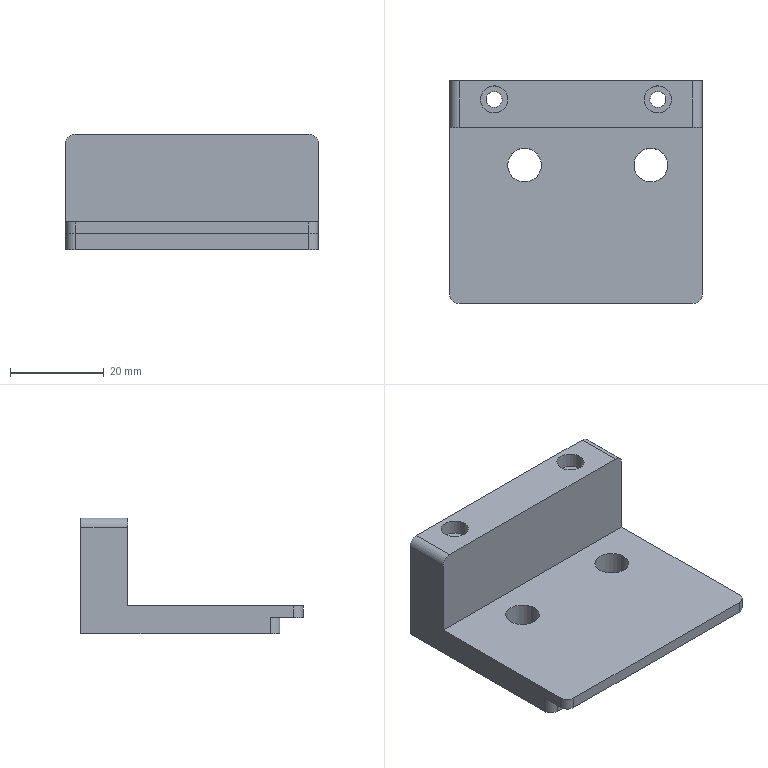Part | STEP file | ROTATION MC_NEW VER-0610_555 | 1 solid | 30 faces | box 54 x 47.54 x 24.76 mm | volume 18101 mm3 | plane 16 | cylinder 14 | commonest cylinder face diameters 4 x6 3 x2 3.4 x2 5.8 x2 7.2 x2
STEP:
#1=CARTESIAN_POINT('',(191.531,578.728,-33.351));
#2=VERTEX_POINT('',#1);
#3=CARTESIAN_POINT('',(193.531,576.728,-33.351));
#4=VERTEX_POINT('',#3);
#5=CARTESIAN_POINT('',(193.531,578.728,-33.351));
#6=DIRECTION('',(0.,0.,1.));
#7=DIRECTION('',(1.,0.,0.));
#8=AXIS2_PLACEMENT_3D('',#5,#6,#7);
#9=CIRCLE('',#8,2.);
#10=EDGE_CURVE('',#2,#4,#9,.T.);
#11=ORIENTED_EDGE('',*,*,#10,.F.);
#12=CARTESIAN_POINT('',(191.531,578.728,-35.851));
#13=VERTEX_POINT('',#12);
#14=CARTESIAN_POINT('',(191.531,578.728,-35.851));
#15=DIRECTION('',(0.,0.,1.));
#16=VECTOR('',#15,2.5);
#17=LINE('',#14,#16);
#18=EDGE_CURVE('',#13,#2,#17,.T.);
#19=ORIENTED_EDGE('',*,*,#18,.F.);
#20=CARTESIAN_POINT('',(193.531,576.728,-35.851));
#21=VERTEX_POINT('',#20);
#22=CARTESIAN_POINT('',(193.531,578.728,-35.851));
#23=DIRECTION('',(0.,0.,-1.));
#24=DIRECTION('',(1.,0.,0.));
#25=AXIS2_PLACEMENT_3D('',#22,#23,#24);
#26=CIRCLE('',#25,2.);
#27=EDGE_CURVE('',#21,#13,#26,.T.);
#28=ORIENTED_EDGE('',*,*,#27,.F.);
#29=CARTESIAN_POINT('',(193.531,576.728,-33.351));
#30=DIRECTION('',(0.,0.,-1.));
#31=VECTOR('',#30,2.5);
#32=LINE('',#29,#31);
#33=EDGE_CURVE('',#4,#21,#32,.T.);
#34=ORIENTED_EDGE('',*,*,#33,.F.);
#35=EDGE_LOOP('',(#11,#19,#28,#34));
#36=FACE_OUTER_BOUND('',#35,.T.);
#37=CARTESIAN_POINT('',(193.531,578.728,-37.851));
#38=DIRECTION('',(0.,0.,1.));
#39=DIRECTION('',(1.,0.,0.));
#40=AXIS2_PLACEMENT_3D('',#37,#38,#39);
#41=CYLINDRICAL_SURFACE('',#40,2.);
#42=ADVANCED_FACE('',(#36),#41,.T.);
#43=CARTESIAN_POINT('',(191.531,583.728,-35.851));
#44=VERTEX_POINT('',#43);
#45=CARTESIAN_POINT('',(193.531,581.728,-35.851));
#46=VERTEX_POINT('',#45);
#47=CARTESIAN_POINT('',(193.531,583.728,-35.851));
#48=DIRECTION('',(0.,0.,1.));
#49=DIRECTION('',(1.,0.,0.));
#50=AXIS2_PLACEMENT_3D('',#47,#48,#49);
#51=CIRCLE('',#50,2.);
#52=EDGE_CURVE('',#44,#46,#51,.T.);
#53=ORIENTED_EDGE('',*,*,#52,.F.);
#54=CARTESIAN_POINT('',(191.531,583.728,-39.351));
#55=VERTEX_POINT('',#54);
#56=CARTESIAN_POINT('',(191.531,583.728,-39.351));
#57=DIRECTION('',(0.,0.,1.));
#58=VECTOR('',#57,3.5);
#59=LINE('',#56,#58);
#60=EDGE_CURVE('',#55,#44,#59,.T.);
#61=ORIENTED_EDGE('',*,*,#60,.F.);
#62=CARTESIAN_POINT('',(193.531,581.728,-39.351));
#63=VERTEX_POINT('',#62);
#64=CARTESIAN_POINT('',(193.531,583.728,-39.351));
#65=DIRECTION('',(0.,0.,-1.));
#66=DIRECTION('',(-1.,0.,0.));
#67=AXIS2_PLACEMENT_3D('',#64,#65,#66);
#68=CIRCLE('',#67,2.);
#69=EDGE_CURVE('',#63,#55,#68,.T.);
#70=ORIENTED_EDGE('',*,*,#69,.F.);
#71=CARTESIAN_POINT('',(193.531,581.728,-35.851));
#72=DIRECTION('',(0.,0.,-1.));
#73=VECTOR('',#72,3.5);
#74=LINE('',#71,#73);
#75=EDGE_CURVE('',#46,#63,#74,.T.);
#76=ORIENTED_EDGE('',*,*,#75,.F.);
#77=EDGE_LOOP('',(#53,#61,#70,#76));
#78=FACE_OUTER_BOUND('',#77,.T.);
#79=CARTESIAN_POINT('',(193.531,583.728,-37.851));
#80=DIRECTION('',(0.,0.,1.));
#81=DIRECTION('',(1.,0.,0.));
#82=AXIS2_PLACEMENT_3D('',#79,#80,#81);
#83=CYLINDRICAL_SURFACE('',#82,2.);
#84=ADVANCED_FACE('',(#78),#83,.T.);
#85=CARTESIAN_POINT('',(243.531,581.728,-35.851));
#86=VERTEX_POINT('',#85);
#87=CARTESIAN_POINT('',(245.531,583.728,-35.851));
#88=VERTEX_POINT('',#87);
#89=CARTESIAN_POINT('',(243.531,583.728,-35.851));
#90=DIRECTION('',(0.,0.,1.));
#91=DIRECTION('',(1.,0.,0.));
#92=AXIS2_PLACEMENT_3D('',#89,#90,#91);
#93=CIRCLE('',#92,2.);
#94=EDGE_CURVE('',#86,#88,#93,.T.);
#95=ORIENTED_EDGE('',*,*,#94,.F.);
#96=CARTESIAN_POINT('',(243.531,581.728,-39.351));
#97=VERTEX_POINT('',#96);
#98=CARTESIAN_POINT('',(243.531,581.728,-39.351));
#99=DIRECTION('',(0.,0.,1.));
#100=VECTOR('',#99,3.5);
#101=LINE('',#98,#100);
#102=EDGE_CURVE('',#97,#86,#101,.T.);
#103=ORIENTED_EDGE('',*,*,#102,.F.);
#104=CARTESIAN_POINT('',(245.531,583.728,-39.351));
#105=VERTEX_POINT('',#104);
#106=CARTESIAN_POINT('',(243.531,583.728,-39.351));
#107=DIRECTION('',(0.,0.,-1.));
#108=DIRECTION('',(-1.,0.,0.));
#109=AXIS2_PLACEMENT_3D('',#106,#107,#108);
#110=CIRCLE('',#109,2.);
#111=EDGE_CURVE('',#105,#97,#110,.T.);
#112=ORIENTED_EDGE('',*,*,#111,.F.);
#113=CARTESIAN_POINT('',(245.531,583.728,-35.851));
#114=DIRECTION('',(0.,0.,-1.));
#115=VECTOR('',#114,3.5);
#116=LINE('',#113,#115);
#117=EDGE_CURVE('',#88,#105,#116,.T.);
#118=ORIENTED_EDGE('',*,*,#117,.F.);
#119=EDGE_LOOP('',(#95,#103,#112,#118));
#120=FACE_OUTER_BOUND('',#119,.T.);
#121=CARTESIAN_POINT('',(243.531,583.728,-17.301));
#122=DIRECTION('',(0.,0.,1.));
#123=DIRECTION('',(1.,0.,0.));
#124=AXIS2_PLACEMENT_3D('',#121,#122,#123);
#125=CYLINDRICAL_SURFACE('',#124,2.);
#126=ADVANCED_FACE('',(#120),#125,.T.);
#127=CARTESIAN_POINT('',(245.531,578.728,-35.851));
#128=VERTEX_POINT('',#127);
#129=CARTESIAN_POINT('',(243.531,576.728,-35.851));
#130=VERTEX_POINT('',#129);
#131=CARTESIAN_POINT('',(243.531,578.728,-35.851));
#132=DIRECTION('',(0.,0.,-1.));
#133=DIRECTION('',(1.,0.,0.));
#134=AXIS2_PLACEMENT_3D('',#131,#132,#133);
#135=CIRCLE('',#134,2.);
#136=EDGE_CURVE('',#128,#130,#135,.T.);
#137=ORIENTED_EDGE('',*,*,#136,.F.);
#138=CARTESIAN_POINT('',(245.531,578.728,-33.351));
#139=VERTEX_POINT('',#138);
#140=CARTESIAN_POINT('',(245.531,578.728,-33.351));
#141=DIRECTION('',(0.,0.,-1.));
#142=VECTOR('',#141,2.5);
#143=LINE('',#140,#142);
#144=EDGE_CURVE('',#139,#128,#143,.T.);
#145=ORIENTED_EDGE('',*,*,#144,.F.);
#146=CARTESIAN_POINT('',(243.531,576.728,-33.351));
#147=VERTEX_POINT('',#146);
#148=CARTESIAN_POINT('',(243.531,578.728,-33.351));
#149=DIRECTION('',(0.,0.,1.));
#150=DIRECTION('',(1.,0.,0.));
#151=AXIS2_PLACEMENT_3D('',#148,#149,#150);
#152=CIRCLE('',#151,2.);
#153=EDGE_CURVE('',#147,#139,#152,.T.);
#154=ORIENTED_EDGE('',*,*,#153,.F.);
#155=CARTESIAN_POINT('',(243.531,576.728,-35.851));
#156=DIRECTION('',(0.,0.,1.));
#157=VECTOR('',#156,2.5);
#158=LINE('',#155,#157);
#159=EDGE_CURVE('',#130,#147,#158,.T.);
#160=ORIENTED_EDGE('',*,*,#159,.F.);
#161=EDGE_LOOP('',(#137,#145,#154,#160));
#162=FACE_OUTER_BOUND('',#161,.T.);
#163=CARTESIAN_POINT('',(243.531,578.728,-37.851));
#164=DIRECTION('',(0.,0.,-1.));
#165=DIRECTION('',(-1.,0.,0.));
#166=AXIS2_PLACEMENT_3D('',#163,#164,#165);
#167=CYLINDRICAL_SURFACE('',#166,2.);
#168=ADVANCED_FACE('',(#162),#167,.T.);
#169=CARTESIAN_POINT('',(237.581,620.967,-23.351));
#170=VERTEX_POINT('',#169);
#171=CARTESIAN_POINT('',(236.031,621.968,-23.351));
#172=VERTEX_POINT('',#171);
#173=CARTESIAN_POINT('',(236.031,620.268,-23.351));
#174=DIRECTION('',(0.,0.,1.));
#175=DIRECTION('',(0.,1.,0.));
#176=AXIS2_PLACEMENT_3D('',#173,#174,#175);
#177=CIRCLE('',#176,1.7);
#178=EDGE_CURVE('',#170,#172,#177,.T.);
#179=ORIENTED_EDGE('',*,*,#178,.F.);
#180=CARTESIAN_POINT('',(237.581,619.57,-23.351));
#181=VERTEX_POINT('',#180);
#182=CARTESIAN_POINT('',(237.581,619.57,-23.351));
#183=CARTESIAN_POINT('',(237.581,619.57,-23.275));
#184=CARTESIAN_POINT('',(237.587,619.584,-23.193));
#185=CARTESIAN_POINT('',(237.611,619.64,-23.043));
#186=CARTESIAN_POINT('',(237.628,619.683,-22.974));
#187=CARTESIAN_POINT('',(237.66,619.78,-22.868));
#188=CARTESIAN_POINT('',(237.678,619.845,-22.818));
#189=CARTESIAN_POINT('',(237.703,619.957,-22.758));
#190=CARTESIAN_POINT('',(237.713,620.018,-22.734));
#191=CARTESIAN_POINT('',(237.727,620.143,-22.704));
#192=CARTESIAN_POINT('',(237.731,620.208,-22.697));
#193=CARTESIAN_POINT('',(237.731,620.328,-22.697));
#194=CARTESIAN_POINT('',(237.727,620.393,-22.704));
#195=CARTESIAN_POINT('',(237.713,620.519,-22.734));
#196=CARTESIAN_POINT('',(237.703,620.579,-22.758));
#197=CARTESIAN_POINT('',(237.678,620.692,-22.818));
#198=CARTESIAN_POINT('',(237.66,620.757,-22.868));
#199=CARTESIAN_POINT('',(237.628,620.853,-22.974));
#200=CARTESIAN_POINT('',(237.611,620.896,-23.043));
#201=CARTESIAN_POINT('',(237.587,620.953,-23.193));
#202=CARTESIAN_POINT('',(237.581,620.967,-23.275));
#203=CARTESIAN_POINT('',(237.581,620.967,-23.351));
#204=B_SPLINE_CURVE_WITH_KNOTS('',3,(#182,#183,#184,#185,#186,#187,#188,#189,#190,#191,#192,#193,#194,#195,#196,#197,#198,#199,#200,#201,#202,#203),.UNSPECIFIED.,.F.,.F.,(4,2,2,2,2,2,2,2,2,2,4),(-0.4114,-0.3885,-0.3656,-0.3445,-0.3265,-0.3086,-0.2906,-0.2726,-0.2515,-0.2286,-0.2057),.UNSPECIFIED.);
#205=EDGE_CURVE('',#181,#170,#204,.T.);
#206=ORIENTED_EDGE('',*,*,#205,.F.);
#207=CARTESIAN_POINT('',(236.031,620.268,-23.351));
#208=DIRECTION('',(0.,0.,1.));
#209=DIRECTION('',(0.,1.,0.));
#210=AXIS2_PLACEMENT_3D('',#207,#208,#209);
#211=CIRCLE('',#210,1.7);
#212=EDGE_CURVE('',#172,#181,#211,.T.);
#213=ORIENTED_EDGE('',*,*,#212,.F.);
#214=CARTESIAN_POINT('',(236.031,621.968,-17.791));
#215=VERTEX_POINT('',#214);
#216=CARTESIAN_POINT('',(236.031,621.968,-23.351));
#217=DIRECTION('',(0.,0.,1.));
#218=VECTOR('',#217,1.7);
#219=LINE('',#216,#218);
#220=EDGE_CURVE('',#172,#215,#219,.T.);
#221=ORIENTED_EDGE('',*,*,#220,.T.);
#222=CARTESIAN_POINT('',(236.031,620.268,-17.791));
#223=DIRECTION('',(0.,0.,-1.));
#224=DIRECTION('',(0.,-1.,0.));
#225=AXIS2_PLACEMENT_3D('',#222,#223,#224);
#226=CIRCLE('',#225,1.7);
#227=EDGE_CURVE('',#215,#215,#226,.T.);
#228=ORIENTED_EDGE('',*,*,#227,.F.);
#229=ORIENTED_EDGE('',*,*,#220,.F.);
#230=EDGE_LOOP('',(#179,#206,#213,#221,#228,#229));
#231=FACE_OUTER_BOUND('',#230,.T.);
#232=CARTESIAN_POINT('',(236.031,620.268,-23.351));
#233=DIRECTION('',(0.,0.,1.));
#234=DIRECTION('',(0.,-1.,0.));
#235=AXIS2_PLACEMENT_3D('',#232,#233,#234);
#236=CYLINDRICAL_SURFACE('',#235,1.7);
#237=ADVANCED_FACE('',(#231),#236,.F.);
#238=CARTESIAN_POINT('',(201.031,617.368,-17.791));
#239=VERTEX_POINT('',#238);
#240=CARTESIAN_POINT('',(201.031,623.168,-17.791));
#241=VERTEX_POINT('',#240);
#242=CARTESIAN_POINT('',(201.031,620.268,-17.791));
#243=DIRECTION('',(0.,0.,1.));
#244=DIRECTION('',(0.,-1.,0.));
#245=AXIS2_PLACEMENT_3D('',#242,#243,#244);
#246=CIRCLE('',#245,2.9);
#247=EDGE_CURVE('',#239,#241,#246,.T.);
#248=ORIENTED_EDGE('',*,*,#247,.T.);
#249=CARTESIAN_POINT('',(201.031,620.268,-17.791));
#250=DIRECTION('',(0.,0.,1.));
#251=DIRECTION('',(0.,-1.,0.));
#252=AXIS2_PLACEMENT_3D('',#249,#250,#251);
#253=CIRCLE('',#252,2.9);
#254=EDGE_CURVE('',#241,#239,#253,.T.);
#255=ORIENTED_EDGE('',*,*,#254,.T.);
#256=EDGE_LOOP('',(#248,#255));
#257=FACE_OUTER_BOUND('',#256,.T.);
#258=CARTESIAN_POINT('',(201.031,618.568,-17.791));
#259=VERTEX_POINT('',#258);
#260=CARTESIAN_POINT('',(201.031,621.968,-17.791));
#261=VERTEX_POINT('',#260);
#262=CARTESIAN_POINT('',(201.031,620.268,-17.791));
#263=DIRECTION('',(0.,0.,-1.));
#264=DIRECTION('',(0.,-1.,0.));
#265=AXIS2_PLACEMENT_3D('',#262,#263,#264);
#266=CIRCLE('',#265,1.7);
#267=EDGE_CURVE('',#259,#261,#266,.T.);
#268=ORIENTED_EDGE('',*,*,#267,.T.);
#269=CARTESIAN_POINT('',(201.031,620.268,-17.791));
#270=DIRECTION('',(0.,0.,-1.));
#271=DIRECTION('',(0.,-1.,0.));
#272=AXIS2_PLACEMENT_3D('',#269,#270,#271);
#273=CIRCLE('',#272,1.7);
#274=EDGE_CURVE('',#261,#259,#273,.T.);
#275=ORIENTED_EDGE('',*,*,#274,.T.);
#276=EDGE_LOOP('',(#268,#275));
#277=FACE_BOUND('',#276,.T.);
#278=CARTESIAN_POINT('',(201.031,621.968,-17.791));
#279=DIRECTION('',(0.,0.,1.));
#280=DIRECTION('',(1.,0.,0.));
#281=AXIS2_PLACEMENT_3D('',#278,#279,#280);
#282=PLANE('',#281);
#283=ADVANCED_FACE('',(#257,#277),#282,.T.);
#284=CARTESIAN_POINT('',(236.031,617.368,-17.791));
#285=VERTEX_POINT('',#284);
#286=CARTESIAN_POINT('',(236.031,623.168,-17.791));
#287=VERTEX_POINT('',#286);
#288=CARTESIAN_POINT('',(236.031,620.268,-17.791));
#289=DIRECTION('',(0.,0.,1.));
#290=DIRECTION('',(0.,-1.,0.));
#291=AXIS2_PLACEMENT_3D('',#288,#289,#290);
#292=CIRCLE('',#291,2.9);
#293=EDGE_CURVE('',#285,#287,#292,.T.);
#294=ORIENTED_EDGE('',*,*,#293,.T.);
#295=CARTESIAN_POINT('',(236.031,620.268,-17.791));
#296=DIRECTION('',(0.,0.,1.));
#297=DIRECTION('',(0.,-1.,0.));
#298=AXIS2_PLACEMENT_3D('',#295,#296,#297);
#299=CIRCLE('',#298,2.9);
#300=EDGE_CURVE('',#287,#285,#299,.T.);
#301=ORIENTED_EDGE('',*,*,#300,.T.);
#302=EDGE_LOOP('',(#294,#301));
#303=FACE_OUTER_BOUND('',#302,.T.);
#304=ORIENTED_EDGE('',*,*,#227,.T.);
#305=EDGE_LOOP('',(#304));
#306=FACE_BOUND('',#305,.T.);
#307=CARTESIAN_POINT('',(236.031,621.968,-17.791));
#308=DIRECTION('',(0.,0.,1.));
#309=DIRECTION('',(1.,0.,0.));
#310=AXIS2_PLACEMENT_3D('',#307,#308,#309);
#311=PLANE('',#310);
#312=ADVANCED_FACE('',(#303,#306),#311,.T.);
#313=ORIENTED_EDGE('',*,*,#293,.F.);
#314=ORIENTED_EDGE('',*,*,#300,.F.);
#315=CARTESIAN_POINT('',(236.031,623.168,-14.591));
#316=VERTEX_POINT('',#315);
#317=CARTESIAN_POINT('',(236.031,623.168,-23.351));
#318=DIRECTION('',(0.,0.,1.));
#319=VECTOR('',#318,2.9);
#320=LINE('',#317,#319);
#321=EDGE_CURVE('',#287,#316,#320,.T.);
#322=ORIENTED_EDGE('',*,*,#321,.T.);
#323=CARTESIAN_POINT('',(236.031,617.368,-14.591));
#324=VERTEX_POINT('',#323);
#325=CARTESIAN_POINT('',(236.031,620.268,-14.591));
#326=DIRECTION('',(0.,0.,-1.));
#327=DIRECTION('',(0.,1.,0.));
#328=AXIS2_PLACEMENT_3D('',#325,#326,#327);
#329=CIRCLE('',#328,2.9);
#330=EDGE_CURVE('',#324,#316,#329,.T.);
#331=ORIENTED_EDGE('',*,*,#330,.F.);
#332=CARTESIAN_POINT('',(236.031,620.268,-14.591));
#333=DIRECTION('',(0.,0.,-1.));
#334=DIRECTION('',(0.,1.,0.));
#335=AXIS2_PLACEMENT_3D('',#332,#333,#334);
#336=CIRCLE('',#335,2.9);
#337=EDGE_CURVE('',#316,#324,#336,.T.);
#338=ORIENTED_EDGE('',*,*,#337,.F.);
#339=ORIENTED_EDGE('',*,*,#321,.F.);
#340=EDGE_LOOP('',(#313,#314,#322,#331,#338,#339));
#341=FACE_OUTER_BOUND('',#340,.T.);
#342=CARTESIAN_POINT('',(236.031,620.268,-23.351));
#343=DIRECTION('',(0.,0.,1.));
#344=DIRECTION('',(0.,-1.,0.));
#345=AXIS2_PLACEMENT_3D('',#342,#343,#344);
#346=CYLINDRICAL_SURFACE('',#345,2.9);
#347=ADVANCED_FACE('',(#341),#346,.F.);
#348=CARTESIAN_POINT('',(199.481,619.57,-23.351));
#349=VERTEX_POINT('',#348);
#350=CARTESIAN_POINT('',(201.031,621.968,-23.351));
#351=VERTEX_POINT('',#350);
#352=CARTESIAN_POINT('',(201.031,620.268,-23.351));
#353=DIRECTION('',(0.,0.,1.));
#354=DIRECTION('',(-0.9118,-0.4107,0.));
#355=AXIS2_PLACEMENT_3D('',#352,#353,#354);
#356=CIRCLE('',#355,1.7);
#357=EDGE_CURVE('',#349,#351,#356,.T.);
#358=ORIENTED_EDGE('',*,*,#357,.F.);
#359=CARTESIAN_POINT('',(199.481,620.967,-23.351));
#360=VERTEX_POINT('',#359);
#361=CARTESIAN_POINT('',(199.481,620.967,-23.351));
#362=CARTESIAN_POINT('',(199.481,620.967,-23.275));
#363=CARTESIAN_POINT('',(199.474,620.953,-23.193));
#364=CARTESIAN_POINT('',(199.451,620.896,-23.043));
#365=CARTESIAN_POINT('',(199.434,620.853,-22.974));
#366=CARTESIAN_POINT('',(199.402,620.757,-22.868));
#367=CARTESIAN_POINT('',(199.383,620.692,-22.818));
#368=CARTESIAN_POINT('',(199.359,620.579,-22.758));
#369=CARTESIAN_POINT('',(199.348,620.519,-22.734));
#370=CARTESIAN_POINT('',(199.334,620.393,-22.704));
#371=CARTESIAN_POINT('',(199.331,620.328,-22.697));
#372=CARTESIAN_POINT('',(199.331,620.208,-22.697));
#373=CARTESIAN_POINT('',(199.334,620.143,-22.704));
#374=CARTESIAN_POINT('',(199.348,620.018,-22.734));
#375=CARTESIAN_POINT('',(199.359,619.957,-22.758));
#376=CARTESIAN_POINT('',(199.383,619.845,-22.818));
#377=CARTESIAN_POINT('',(199.402,619.78,-22.868));
#378=CARTESIAN_POINT('',(199.434,619.683,-22.974));
#379=CARTESIAN_POINT('',(199.451,619.64,-23.043));
#380=CARTESIAN_POINT('',(199.474,619.584,-23.193));
#381=CARTESIAN_POINT('',(199.481,619.57,-23.275));
#382=CARTESIAN_POINT('',(199.481,619.57,-23.351));
#383=B_SPLINE_CURVE_WITH_KNOTS('',3,(#361,#362,#363,#364,#365,#366,#367,#368,#369,#370,#371,#372,#373,#374,#375,#376,#377,#378,#379,#380,#381,#382),.UNSPECIFIED.,.F.,.F.,(4,2,2,2,2,2,2,2,2,2,4),(-0.4114,-0.3885,-0.3656,-0.3445,-0.3265,-0.3086,-0.2906,-0.2726,-0.2515,-0.2286,-0.2057),.UNSPECIFIED.);
#384=EDGE_CURVE('',#360,#349,#383,.T.);
#385=ORIENTED_EDGE('',*,*,#384,.F.);
#386=CARTESIAN_POINT('',(201.031,620.268,-23.351));
#387=DIRECTION('',(0.,0.,1.));
#388=DIRECTION('',(-0.9118,-0.4107,0.));
#389=AXIS2_PLACEMENT_3D('',#386,#387,#388);
#390=CIRCLE('',#389,1.7);
#391=EDGE_CURVE('',#351,#360,#390,.T.);
#392=ORIENTED_EDGE('',*,*,#391,.F.);
#393=CARTESIAN_POINT('',(201.031,621.968,-23.351));
#394=DIRECTION('',(0.,0.,1.));
#395=VECTOR('',#394,1.7);
#396=LINE('',#393,#395);
#397=EDGE_CURVE('',#351,#261,#396,.T.);
#398=ORIENTED_EDGE('',*,*,#397,.T.);
#399=ORIENTED_EDGE('',*,*,#267,.F.);
#400=ORIENTED_EDGE('',*,*,#274,.F.);
#401=ORIENTED_EDGE('',*,*,#397,.F.);
#402=EDGE_LOOP('',(#358,#385,#392,#398,#399,#400,#401));
#403=FACE_OUTER_BOUND('',#402,.T.);
#404=CARTESIAN_POINT('',(201.031,620.268,-23.351));
#405=DIRECTION('',(0.,0.,1.));
#406=DIRECTION('',(0.,-1.,0.));
#407=AXIS2_PLACEMENT_3D('',#404,#405,#406);
#408=CYLINDRICAL_SURFACE('',#407,1.7);
#409=ADVANCED_FACE('',(#403),#408,.F.);
#410=CARTESIAN_POINT('',(243.531,624.268,-14.591));
#411=VERTEX_POINT('',#410);
#412=CARTESIAN_POINT('',(243.531,614.268,-14.591));
#413=VERTEX_POINT('',#412);
#414=CARTESIAN_POINT('',(243.531,624.268,-14.591));
#415=DIRECTION('',(0.,-1.,0.));
#416=VECTOR('',#415,10.);
#417=LINE('',#414,#416);
#418=EDGE_CURVE('',#411,#413,#417,.T.);
#419=ORIENTED_EDGE('',*,*,#418,.F.);
#420=CARTESIAN_POINT('',(193.531,624.268,-14.591));
#421=VERTEX_POINT('',#420);
#422=CARTESIAN_POINT('',(193.531,624.268,-14.591));
#423=DIRECTION('',(1.,0.,0.));
#424=VECTOR('',#423,50.);
#425=LINE('',#422,#424);
#426=EDGE_CURVE('',#421,#411,#425,.T.);
#427=ORIENTED_EDGE('',*,*,#426,.F.);
#428=CARTESIAN_POINT('',(193.531,614.268,-14.591));
#429=VERTEX_POINT('',#428);
#430=CARTESIAN_POINT('',(193.531,614.268,-14.591));
#431=DIRECTION('',(0.,1.,0.));
#432=VECTOR('',#431,10.);
#433=LINE('',#430,#432);
#434=EDGE_CURVE('',#429,#421,#433,.T.);
#435=ORIENTED_EDGE('',*,*,#434,.F.);
#436=CARTESIAN_POINT('',(243.531,614.268,-14.591));
#437=DIRECTION('',(-1.,0.,0.));
#438=VECTOR('',#437,50.);
#439=LINE('',#436,#438);
#440=EDGE_CURVE('',#413,#429,#439,.T.);
#441=ORIENTED_EDGE('',*,*,#440,.F.);
#442=EDGE_LOOP('',(#419,#427,#435,#441));
#443=FACE_OUTER_BOUND('',#442,.T.);
#444=CARTESIAN_POINT('',(201.031,617.368,-14.591));
#445=VERTEX_POINT('',#444);
#446=CARTESIAN_POINT('',(201.031,623.168,-14.591));
#447=VERTEX_POINT('',#446);
#448=CARTESIAN_POINT('',(201.031,620.268,-14.591));
#449=DIRECTION('',(0.,0.,-1.));
#450=DIRECTION('',(0.,-1.,0.));
#451=AXIS2_PLACEMENT_3D('',#448,#449,#450);
#452=CIRCLE('',#451,2.9);
#453=EDGE_CURVE('',#445,#447,#452,.T.);
#454=ORIENTED_EDGE('',*,*,#453,.T.);
#455=CARTESIAN_POINT('',(201.031,620.268,-14.591));
#456=DIRECTION('',(0.,0.,-1.));
#457=DIRECTION('',(0.,-1.,0.));
#458=AXIS2_PLACEMENT_3D('',#455,#456,#457);
#459=CIRCLE('',#458,2.9);
#460=EDGE_CURVE('',#447,#445,#459,.T.);
#461=ORIENTED_EDGE('',*,*,#460,.T.);
#462=EDGE_LOOP('',(#454,#461));
#463=FACE_BOUND('',#462,.T.);
#464=ORIENTED_EDGE('',*,*,#330,.T.);
#465=ORIENTED_EDGE('',*,*,#337,.T.);
#466=EDGE_LOOP('',(#464,#465));
#467=FACE_BOUND('',#466,.T.);
#468=CARTESIAN_POINT('',(211.031,593.728,-14.591));
#469=DIRECTION('',(0.,0.,1.));
#470=DIRECTION('',(1.,0.,0.));
#471=AXIS2_PLACEMENT_3D('',#468,#469,#470);
#472=PLANE('',#471);
#473=ADVANCED_FACE('',(#443,#463,#467),#472,.T.);
#474=CARTESIAN_POINT('',(245.531,614.268,-16.591));
#475=VERTEX_POINT('',#474);
#476=CARTESIAN_POINT('',(243.531,614.268,-16.591));
#477=DIRECTION('',(0.,-1.,0.));
#478=DIRECTION('',(0.7071,0.,0.7071));
#479=AXIS2_PLACEMENT_3D('',#476,#477,#478);
#480=CIRCLE('',#479,2.);
#481=EDGE_CURVE('',#475,#413,#480,.T.);
#482=ORIENTED_EDGE('',*,*,#481,.F.);
#483=CARTESIAN_POINT('',(245.531,624.268,-16.591));
#484=VERTEX_POINT('',#483);
#485=CARTESIAN_POINT('',(245.531,614.268,-16.591));
#486=DIRECTION('',(0.,1.,0.));
#487=VECTOR('',#486,10.);
#488=LINE('',#485,#487);
#489=EDGE_CURVE('',#475,#484,#488,.T.);
#490=ORIENTED_EDGE('',*,*,#489,.T.);
#491=CARTESIAN_POINT('',(243.531,624.268,-16.591));
#492=DIRECTION('',(0.,1.,0.));
#493=DIRECTION('',(0.,0.,1.));
#494=AXIS2_PLACEMENT_3D('',#491,#492,#493);
#495=CIRCLE('',#494,2.);
#496=EDGE_CURVE('',#411,#484,#495,.T.);
#497=ORIENTED_EDGE('',*,*,#496,.F.);
#498=ORIENTED_EDGE('',*,*,#418,.T.);
#499=EDGE_LOOP('',(#482,#490,#497,#498));
#500=FACE_OUTER_BOUND('',#499,.T.);
#501=CARTESIAN_POINT('',(243.531,593.728,-16.591));
#502=DIRECTION('',(0.,1.,0.));
#503=DIRECTION('',(0.7071,0.,0.7071));
#504=AXIS2_PLACEMENT_3D('',#501,#502,#503);
#505=CYLINDRICAL_SURFACE('',#504,2.);
#506=ADVANCED_FACE('',(#500),#505,.T.);
#507=CARTESIAN_POINT('',(199.481,624.268,-23.351));
#508=VERTEX_POINT('',#507);
#509=CARTESIAN_POINT('',(199.481,624.268,-23.351));
#510=DIRECTION('',(0.,-1.,0.));
#511=VECTOR('',#510,3.302);
#512=LINE('',#509,#511);
#513=EDGE_CURVE('',#508,#360,#512,.T.);
#514=ORIENTED_EDGE('',*,*,#513,.F.);
#515=CARTESIAN_POINT('',(237.581,624.268,-23.351));
#516=VERTEX_POINT('',#515);
#517=CARTESIAN_POINT('',(199.481,624.268,-23.351));
#518=DIRECTION('',(1.,0.,0.));
#519=VECTOR('',#518,38.1);
#520=LINE('',#517,#519);
#521=EDGE_CURVE('',#508,#516,#520,.T.);
#522=ORIENTED_EDGE('',*,*,#521,.T.);
#523=CARTESIAN_POINT('',(237.581,620.967,-23.351));
#524=DIRECTION('',(0.,1.,0.));
#525=VECTOR('',#524,3.302);
#526=LINE('',#523,#525);
#527=EDGE_CURVE('',#170,#516,#526,.T.);
#528=ORIENTED_EDGE('',*,*,#527,.F.);
#529=ORIENTED_EDGE('',*,*,#178,.T.);
#530=ORIENTED_EDGE('',*,*,#212,.T.);
#531=CARTESIAN_POINT('',(237.581,616.268,-23.351));
#532=VERTEX_POINT('',#531);
#533=CARTESIAN_POINT('',(237.581,616.268,-23.351));
#534=DIRECTION('',(0.,1.,0.));
#535=VECTOR('',#534,3.302);
#536=LINE('',#533,#535);
#537=EDGE_CURVE('',#532,#181,#536,.T.);
#538=ORIENTED_EDGE('',*,*,#537,.F.);
#539=CARTESIAN_POINT('',(199.481,616.268,-23.351));
#540=VERTEX_POINT('',#539);
#541=CARTESIAN_POINT('',(199.481,616.268,-23.351));
#542=DIRECTION('',(1.,0.,0.));
#543=VECTOR('',#542,38.1);
#544=LINE('',#541,#543);
#545=EDGE_CURVE('',#540,#532,#544,.T.);
#546=ORIENTED_EDGE('',*,*,#545,.F.);
#547=CARTESIAN_POINT('',(199.481,619.57,-23.351));
#548=DIRECTION('',(0.,-1.,0.));
#549=VECTOR('',#548,3.302);
#550=LINE('',#547,#549);
#551=EDGE_CURVE('',#349,#540,#550,.T.);
#552=ORIENTED_EDGE('',*,*,#551,.F.);
#553=ORIENTED_EDGE('',*,*,#357,.T.);
#554=ORIENTED_EDGE('',*,*,#391,.T.);
#555=EDGE_LOOP('',(#514,#522,#528,#529,#530,#538,#546,#552,#553,#554));
#556=FACE_OUTER_BOUND('',#555,.T.);
#557=CARTESIAN_POINT('',(211.031,593.728,-23.351));
#558=DIRECTION('',(0.,0.,-1.));
#559=DIRECTION('',(-1.,0.,0.));
#560=AXIS2_PLACEMENT_3D('',#557,#558,#559);
#561=PLANE('',#560);
#562=ADVANCED_FACE('',(#556),#561,.T.);
#563=ORIENTED_EDGE('',*,*,#496,.T.);
#564=CARTESIAN_POINT('',(245.531,624.268,-39.351));
#565=VERTEX_POINT('',#564);
#566=CARTESIAN_POINT('',(245.531,624.268,-16.591));
#567=DIRECTION('',(0.,0.,-1.));
#568=VECTOR('',#567,22.76);
#569=LINE('',#566,#568);
#570=EDGE_CURVE('',#484,#565,#569,.T.);
#571=ORIENTED_EDGE('',*,*,#570,.T.);
#572=CARTESIAN_POINT('',(240.581,624.268,-39.351));
#573=VERTEX_POINT('',#572);
#574=CARTESIAN_POINT('',(245.531,624.268,-39.351));
#575=DIRECTION('',(-1.,0.,0.));
#576=VECTOR('',#575,4.95);
#577=LINE('',#574,#576);
#578=EDGE_CURVE('',#565,#573,#577,.T.);
#579=ORIENTED_EDGE('',*,*,#578,.T.);
#580=CARTESIAN_POINT('',(240.581,624.268,-23.351));
#581=VERTEX_POINT('',#580);
#582=CARTESIAN_POINT('',(240.581,624.268,-23.351));
#583=DIRECTION('',(0.,0.,-1.));
#584=VECTOR('',#583,16.);
#585=LINE('',#582,#584);
#586=EDGE_CURVE('',#581,#573,#585,.T.);
#587=ORIENTED_EDGE('',*,*,#586,.F.);
#588=CARTESIAN_POINT('',(239.081,624.268,-23.351));
#589=DIRECTION('',(0.,-1.,0.));
#590=DIRECTION('',(1.,0.,0.));
#591=AXIS2_PLACEMENT_3D('',#588,#589,#590);
#592=CIRCLE('',#591,1.5);
#593=EDGE_CURVE('',#581,#516,#592,.T.);
#594=ORIENTED_EDGE('',*,*,#593,.T.);
#595=ORIENTED_EDGE('',*,*,#521,.F.);
#596=CARTESIAN_POINT('',(196.481,624.268,-23.351));
#597=VERTEX_POINT('',#596);
#598=CARTESIAN_POINT('',(197.981,624.268,-23.351));
#599=DIRECTION('',(0.,-1.,0.));
#600=DIRECTION('',(1.,0.,0.));
#601=AXIS2_PLACEMENT_3D('',#598,#599,#600);
#602=CIRCLE('',#601,1.5);
#603=EDGE_CURVE('',#508,#597,#602,.T.);
#604=ORIENTED_EDGE('',*,*,#603,.T.);
#605=CARTESIAN_POINT('',(196.481,624.268,-39.351));
#606=VERTEX_POINT('',#605);
#607=CARTESIAN_POINT('',(196.481,624.268,-39.351));
#608=DIRECTION('',(0.,0.,1.));
#609=VECTOR('',#608,16.);
#610=LINE('',#607,#609);
#611=EDGE_CURVE('',#606,#597,#610,.T.);
#612=ORIENTED_EDGE('',*,*,#611,.F.);
#613=CARTESIAN_POINT('',(191.531,624.268,-39.351));
#614=VERTEX_POINT('',#613);
#615=CARTESIAN_POINT('',(196.481,624.268,-39.351));
#616=DIRECTION('',(-1.,0.,0.));
#617=VECTOR('',#616,4.95);
#618=LINE('',#615,#617);
#619=EDGE_CURVE('',#606,#614,#618,.T.);
#620=ORIENTED_EDGE('',*,*,#619,.T.);
#621=CARTESIAN_POINT('',(191.531,624.268,-16.591));
#622=VERTEX_POINT('',#621);
#623=CARTESIAN_POINT('',(191.531,624.268,-16.591));
#624=DIRECTION('',(0.,0.,-1.));
#625=VECTOR('',#624,22.76);
#626=LINE('',#623,#625);
#627=EDGE_CURVE('',#622,#614,#626,.T.);
#628=ORIENTED_EDGE('',*,*,#627,.F.);
#629=CARTESIAN_POINT('',(193.531,624.268,-16.591));
#630=DIRECTION('',(0.,1.,0.));
#631=DIRECTION('',(-1.,0.,0.));
#632=AXIS2_PLACEMENT_3D('',#629,#630,#631);
#633=CIRCLE('',#632,2.);
#634=EDGE_CURVE('',#622,#421,#633,.T.);
#635=ORIENTED_EDGE('',*,*,#634,.T.);
#636=ORIENTED_EDGE('',*,*,#426,.T.);
#637=EDGE_LOOP('',(#563,#571,#579,#587,#594,#595,#604,#612,#620,#628,#635,#636));
#638=FACE_OUTER_BOUND('',#637,.T.);
#639=CARTESIAN_POINT('',(218.531,624.268,-40.291));
#640=DIRECTION('',(0.,1.,0.));
#641=DIRECTION('',(0.,0.,1.));
#642=AXIS2_PLACEMENT_3D('',#639,#640,#641);
#643=PLANE('',#642);
#644=ADVANCED_FACE('',(#638),#643,.T.);
#645=CARTESIAN_POINT('',(191.531,614.268,-16.591));
#646=VERTEX_POINT('',#645);
#647=CARTESIAN_POINT('',(193.531,614.268,-16.591));
#648=DIRECTION('',(0.,-1.,0.));
#649=DIRECTION('',(0.,0.,1.));
#650=AXIS2_PLACEMENT_3D('',#647,#648,#649);
#651=CIRCLE('',#650,2.);
#652=EDGE_CURVE('',#429,#646,#651,.T.);
#653=ORIENTED_EDGE('',*,*,#652,.F.);
#654=ORIENTED_EDGE('',*,*,#434,.T.);
#655=ORIENTED_EDGE('',*,*,#634,.F.);
#656=CARTESIAN_POINT('',(191.531,624.268,-16.591));
#657=DIRECTION('',(0.,-1.,0.));
#658=VECTOR('',#657,10.);
#659=LINE('',#656,#658);
#660=EDGE_CURVE('',#622,#646,#659,.T.);
#661=ORIENTED_EDGE('',*,*,#660,.T.);
#662=EDGE_LOOP('',(#653,#654,#655,#661));
#663=FACE_OUTER_BOUND('',#662,.T.);
#664=CARTESIAN_POINT('',(193.531,593.728,-16.591));
#665=DIRECTION('',(0.,1.,0.));
#666=DIRECTION('',(-0.7071,0.,0.7071));
#667=AXIS2_PLACEMENT_3D('',#664,#665,#666);
#668=CYLINDRICAL_SURFACE('',#667,2.);
#669=ADVANCED_FACE('',(#663),#668,.T.);
#670=ORIENTED_EDGE('',*,*,#611,.T.);
#671=CARTESIAN_POINT('',(196.481,616.268,-23.351));
#672=VERTEX_POINT('',#671);
#673=CARTESIAN_POINT('',(196.481,616.268,-23.351));
#674=DIRECTION('',(0.,1.,0.));
#675=VECTOR('',#674,8.);
#676=LINE('',#673,#675);
#677=EDGE_CURVE('',#672,#597,#676,.T.);
#678=ORIENTED_EDGE('',*,*,#677,.F.);
#679=CARTESIAN_POINT('',(196.481,616.268,-39.351));
#680=VERTEX_POINT('',#679);
#681=CARTESIAN_POINT('',(196.481,616.268,-39.351));
#682=DIRECTION('',(0.,0.,1.));
#683=VECTOR('',#682,16.);
#684=LINE('',#681,#683);
#685=EDGE_CURVE('',#680,#672,#684,.T.);
#686=ORIENTED_EDGE('',*,*,#685,.F.);
#687=CARTESIAN_POINT('',(196.481,624.268,-39.351));
#688=DIRECTION('',(0.,-1.,0.));
#689=VECTOR('',#688,8.);
#690=LINE('',#687,#689);
#691=EDGE_CURVE('',#606,#680,#690,.T.);
#692=ORIENTED_EDGE('',*,*,#691,.F.);
#693=EDGE_LOOP('',(#670,#678,#686,#692));
#694=FACE_OUTER_BOUND('',#693,.T.);
#695=CARTESIAN_POINT('',(196.481,617.268,-23.531));
#696=DIRECTION('',(1.,0.,0.));
#697=DIRECTION('',(0.,0.,-1.));
#698=AXIS2_PLACEMENT_3D('',#695,#696,#697);
#699=PLANE('',#698);
#700=ADVANCED_FACE('',(#694),#699,.T.);
#701=ORIENTED_EDGE('',*,*,#481,.T.);
#702=ORIENTED_EDGE('',*,*,#440,.T.);
#703=ORIENTED_EDGE('',*,*,#652,.T.);
#704=CARTESIAN_POINT('',(191.531,614.268,-33.351));
#705=VERTEX_POINT('',#704);
#706=CARTESIAN_POINT('',(191.531,614.268,-16.591));
#707=DIRECTION('',(0.,0.,-1.));
#708=VECTOR('',#707,16.76);
#709=LINE('',#706,#708);
#710=EDGE_CURVE('',#646,#705,#709,.T.);
#711=ORIENTED_EDGE('',*,*,#710,.T.);
#712=CARTESIAN_POINT('',(245.531,614.268,-33.351));
#713=VERTEX_POINT('',#712);
#714=CARTESIAN_POINT('',(245.531,614.268,-33.351));
#715=DIRECTION('',(-1.,0.,0.));
#716=VECTOR('',#715,54.);
#717=LINE('',#714,#716);
#718=EDGE_CURVE('',#713,#705,#717,.T.);
#719=ORIENTED_EDGE('',*,*,#718,.F.);
#720=CARTESIAN_POINT('',(245.531,614.268,-33.351));
#721=DIRECTION('',(0.,0.,1.));
#722=VECTOR('',#721,16.76);
#723=LINE('',#720,#722);
#724=EDGE_CURVE('',#713,#475,#723,.T.);
#725=ORIENTED_EDGE('',*,*,#724,.T.);
#726=EDGE_LOOP('',(#701,#702,#703,#711,#719,#725));
#727=FACE_OUTER_BOUND('',#726,.T.);
#728=CARTESIAN_POINT('',(218.531,614.268,-23.531));
#729=DIRECTION('',(0.,-1.,0.));
#730=DIRECTION('',(0.,0.,-1.));
#731=AXIS2_PLACEMENT_3D('',#728,#729,#730);
#732=PLANE('',#731);
#733=ADVANCED_FACE('',(#727),#732,.T.);
#734=CARTESIAN_POINT('',(245.531,614.268,-33.351));
#735=DIRECTION('',(0.,-1.,0.));
#736=VECTOR('',#735,35.54);
#737=LINE('',#734,#736);
#738=EDGE_CURVE('',#713,#139,#737,.T.);
#739=ORIENTED_EDGE('',*,*,#738,.T.);
#740=ORIENTED_EDGE('',*,*,#144,.T.);
#741=CARTESIAN_POINT('',(245.531,578.728,-35.851));
#742=DIRECTION('',(0.,1.,0.));
#743=VECTOR('',#742,5.);
#744=LINE('',#741,#743);
#745=EDGE_CURVE('',#128,#88,#744,.T.);
#746=ORIENTED_EDGE('',*,*,#745,.T.);
#747=ORIENTED_EDGE('',*,*,#117,.T.);
#748=CARTESIAN_POINT('',(245.531,624.268,-39.351));
#749=DIRECTION('',(0.,-1.,0.));
#750=VECTOR('',#749,40.54);
#751=LINE('',#748,#750);
#752=EDGE_CURVE('',#565,#105,#751,.T.);
#753=ORIENTED_EDGE('',*,*,#752,.F.);
#754=ORIENTED_EDGE('',*,*,#570,.F.);
#755=ORIENTED_EDGE('',*,*,#489,.F.);
#756=ORIENTED_EDGE('',*,*,#724,.F.);
#757=EDGE_LOOP('',(#739,#740,#746,#747,#753,#754,#755,#756));
#758=FACE_OUTER_BOUND('',#757,.T.);
#759=CARTESIAN_POINT('',(245.531,593.728,-17.301));
#760=DIRECTION('',(1.,0.,0.));
#761=DIRECTION('',(0.,0.,-1.));
#762=AXIS2_PLACEMENT_3D('',#759,#760,#761);
#763=PLANE('',#762);
#764=ADVANCED_FACE('',(#758),#763,.T.);
#765=ORIENTED_EDGE('',*,*,#752,.T.);
#766=ORIENTED_EDGE('',*,*,#111,.T.);
#767=CARTESIAN_POINT('',(243.531,581.728,-39.351));
#768=DIRECTION('',(-1.,0.,0.));
#769=VECTOR('',#768,50.);
#770=LINE('',#767,#769);
#771=EDGE_CURVE('',#97,#63,#770,.T.);
#772=ORIENTED_EDGE('',*,*,#771,.T.);
#773=ORIENTED_EDGE('',*,*,#69,.T.);
#774=CARTESIAN_POINT('',(191.531,624.268,-39.351));
#775=DIRECTION('',(0.,-1.,0.));
#776=VECTOR('',#775,40.54);
#777=LINE('',#774,#776);
#778=EDGE_CURVE('',#614,#55,#777,.T.);
#779=ORIENTED_EDGE('',*,*,#778,.F.);
#780=ORIENTED_EDGE('',*,*,#619,.F.);
#781=ORIENTED_EDGE('',*,*,#691,.T.);
#782=CARTESIAN_POINT('',(240.581,616.268,-39.351));
#783=VERTEX_POINT('',#782);
#784=CARTESIAN_POINT('',(240.581,616.268,-39.351));
#785=DIRECTION('',(-1.,0.,0.));
#786=VECTOR('',#785,44.1);
#787=LINE('',#784,#786);
#788=EDGE_CURVE('',#783,#680,#787,.T.);
#789=ORIENTED_EDGE('',*,*,#788,.F.);
#790=CARTESIAN_POINT('',(240.581,616.268,-39.351));
#791=DIRECTION('',(0.,1.,0.));
#792=VECTOR('',#791,8.);
#793=LINE('',#790,#792);
#794=EDGE_CURVE('',#783,#573,#793,.T.);
#795=ORIENTED_EDGE('',*,*,#794,.T.);
#796=ORIENTED_EDGE('',*,*,#578,.F.);
#797=EDGE_LOOP('',(#765,#766,#772,#773,#779,#780,#781,#789,#795,#796));
#798=FACE_OUTER_BOUND('',#797,.T.);
#799=CARTESIAN_POINT('',(203.931,606.268,-39.351));
#800=VERTEX_POINT('',#799);
#801=CARTESIAN_POINT('',(211.131,606.268,-39.351));
#802=VERTEX_POINT('',#801);
#803=CARTESIAN_POINT('',(207.531,606.268,-39.351));
#804=DIRECTION('',(0.,0.,1.));
#805=DIRECTION('',(-1.,0.,0.));
#806=AXIS2_PLACEMENT_3D('',#803,#804,#805);
#807=CIRCLE('',#806,3.6);
#808=EDGE_CURVE('',#800,#802,#807,.T.);
#809=ORIENTED_EDGE('',*,*,#808,.T.);
#810=CARTESIAN_POINT('',(207.531,606.268,-39.351));
#811=DIRECTION('',(0.,0.,1.));
#812=DIRECTION('',(-1.,0.,0.));
#813=AXIS2_PLACEMENT_3D('',#810,#811,#812);
#814=CIRCLE('',#813,3.6);
#815=EDGE_CURVE('',#802,#800,#814,.T.);
#816=ORIENTED_EDGE('',*,*,#815,.T.);
#817=EDGE_LOOP('',(#809,#816));
#818=FACE_BOUND('',#817,.T.);
#819=CARTESIAN_POINT('',(230.931,606.268,-39.351));
#820=VERTEX_POINT('',#819);
#821=CARTESIAN_POINT('',(238.131,606.268,-39.351));
#822=VERTEX_POINT('',#821);
#823=CARTESIAN_POINT('',(234.531,606.268,-39.351));
#824=DIRECTION('',(0.,0.,1.));
#825=DIRECTION('',(-1.,0.,0.));
#826=AXIS2_PLACEMENT_3D('',#823,#824,#825);
#827=CIRCLE('',#826,3.6);
#828=EDGE_CURVE('',#820,#822,#827,.T.);
#829=ORIENTED_EDGE('',*,*,#828,.T.);
#830=CARTESIAN_POINT('',(234.531,606.268,-39.351));
#831=DIRECTION('',(0.,0.,1.));
#832=DIRECTION('',(-1.,0.,0.));
#833=AXIS2_PLACEMENT_3D('',#830,#831,#832);
#834=CIRCLE('',#833,3.6);
#835=EDGE_CURVE('',#822,#820,#834,.T.);
#836=ORIENTED_EDGE('',*,*,#835,.T.);
#837=EDGE_LOOP('',(#829,#836));
#838=FACE_BOUND('',#837,.T.);
#839=CARTESIAN_POINT('',(211.031,593.728,-39.351));
#840=DIRECTION('',(0.,0.,-1.));
#841=DIRECTION('',(-1.,0.,0.));
#842=AXIS2_PLACEMENT_3D('',#839,#840,#841);
#843=PLANE('',#842);
#844=ADVANCED_FACE('',(#798,#818,#838),#843,.T.);
#845=ORIENTED_EDGE('',*,*,#685,.T.);
#846=CARTESIAN_POINT('',(197.981,616.268,-23.351));
#847=DIRECTION('',(0.,1.,0.));
#848=DIRECTION('',(-1.,0.,0.));
#849=AXIS2_PLACEMENT_3D('',#846,#847,#848);
#850=CIRCLE('',#849,1.5);
#851=EDGE_CURVE('',#672,#540,#850,.T.);
#852=ORIENTED_EDGE('',*,*,#851,.T.);
#853=ORIENTED_EDGE('',*,*,#545,.T.);
#854=CARTESIAN_POINT('',(240.581,616.268,-23.351));
#855=VERTEX_POINT('',#854);
#856=CARTESIAN_POINT('',(239.081,616.268,-23.351));
#857=DIRECTION('',(0.,1.,0.));
#858=DIRECTION('',(-1.,0.,0.));
#859=AXIS2_PLACEMENT_3D('',#856,#857,#858);
#860=CIRCLE('',#859,1.5);
#861=EDGE_CURVE('',#532,#855,#860,.T.);
#862=ORIENTED_EDGE('',*,*,#861,.T.);
#863=CARTESIAN_POINT('',(240.581,616.268,-23.351));
#864=DIRECTION('',(0.,0.,-1.));
#865=VECTOR('',#864,16.);
#866=LINE('',#863,#865);
#867=EDGE_CURVE('',#855,#783,#866,.T.);
#868=ORIENTED_EDGE('',*,*,#867,.T.);
#869=ORIENTED_EDGE('',*,*,#788,.T.);
#870=EDGE_LOOP('',(#845,#852,#853,#862,#868,#869));
#871=FACE_OUTER_BOUND('',#870,.T.);
#872=CARTESIAN_POINT('',(218.531,616.268,-32.531));
#873=DIRECTION('',(0.,-1.,0.));
#874=DIRECTION('',(0.,0.,-1.));
#875=AXIS2_PLACEMENT_3D('',#872,#873,#874);
#876=PLANE('',#875);
#877=ADVANCED_FACE('',(#871),#876,.F.);
#878=ORIENTED_EDGE('',*,*,#745,.F.);
#879=ORIENTED_EDGE('',*,*,#136,.T.);
#880=CARTESIAN_POINT('',(193.531,576.728,-35.851));
#881=DIRECTION('',(1.,0.,0.));
#882=VECTOR('',#881,50.);
#883=LINE('',#880,#882);
#884=EDGE_CURVE('',#21,#130,#883,.T.);
#885=ORIENTED_EDGE('',*,*,#884,.F.);
#886=ORIENTED_EDGE('',*,*,#27,.T.);
#887=CARTESIAN_POINT('',(191.531,583.728,-35.851));
#888=DIRECTION('',(0.,-1.,0.));
#889=VECTOR('',#888,5.);
#890=LINE('',#887,#889);
#891=EDGE_CURVE('',#44,#13,#890,.T.);
#892=ORIENTED_EDGE('',*,*,#891,.F.);
#893=ORIENTED_EDGE('',*,*,#52,.T.);
#894=CARTESIAN_POINT('',(243.531,581.728,-35.851));
#895=DIRECTION('',(-1.,0.,0.));
#896=VECTOR('',#895,50.);
#897=LINE('',#894,#896);
#898=EDGE_CURVE('',#86,#46,#897,.T.);
#899=ORIENTED_EDGE('',*,*,#898,.F.);
#900=ORIENTED_EDGE('',*,*,#94,.T.);
#901=EDGE_LOOP('',(#878,#879,#885,#886,#892,#893,#899,#900));
#902=FACE_OUTER_BOUND('',#901,.T.);
#903=CARTESIAN_POINT('',(292.531,896.728,-35.851));
#904=DIRECTION('',(0.,0.,1.));
#905=DIRECTION('',(1.,0.,0.));
#906=AXIS2_PLACEMENT_3D('',#903,#904,#905);
#907=PLANE('',#906);
#908=ADVANCED_FACE('',(#902),#907,.F.);
#909=ORIENTED_EDGE('',*,*,#677,.T.);
#910=ORIENTED_EDGE('',*,*,#603,.F.);
#911=ORIENTED_EDGE('',*,*,#513,.T.);
#912=ORIENTED_EDGE('',*,*,#384,.T.);
#913=ORIENTED_EDGE('',*,*,#551,.T.);
#914=ORIENTED_EDGE('',*,*,#851,.F.);
#915=EDGE_LOOP('',(#909,#910,#911,#912,#913,#914));
#916=FACE_OUTER_BOUND('',#915,.T.);
#917=CARTESIAN_POINT('',(197.981,624.268,-23.351));
#918=DIRECTION('',(0.,-1.,0.));
#919=DIRECTION('',(1.,0.,0.));
#920=AXIS2_PLACEMENT_3D('',#917,#918,#919);
#921=CYLINDRICAL_SURFACE('',#920,1.5);
#922=ADVANCED_FACE('',(#916),#921,.F.);
#923=CARTESIAN_POINT('',(193.531,576.728,-33.351));
#924=DIRECTION('',(1.,0.,0.));
#925=VECTOR('',#924,50.);
#926=LINE('',#923,#925);
#927=EDGE_CURVE('',#4,#147,#926,.T.);
#928=ORIENTED_EDGE('',*,*,#927,.T.);
#929=ORIENTED_EDGE('',*,*,#153,.T.);
#930=ORIENTED_EDGE('',*,*,#738,.F.);
#931=ORIENTED_EDGE('',*,*,#718,.T.);
#932=CARTESIAN_POINT('',(191.531,614.268,-33.351));
#933=DIRECTION('',(0.,-1.,0.));
#934=VECTOR('',#933,35.54);
#935=LINE('',#932,#934);
#936=EDGE_CURVE('',#705,#2,#935,.T.);
#937=ORIENTED_EDGE('',*,*,#936,.T.);
#938=ORIENTED_EDGE('',*,*,#10,.T.);
#939=EDGE_LOOP('',(#928,#929,#930,#931,#937,#938));
#940=FACE_OUTER_BOUND('',#939,.T.);
#941=CARTESIAN_POINT('',(203.931,606.268,-33.351));
#942=VERTEX_POINT('',#941);
#943=CARTESIAN_POINT('',(211.131,606.268,-33.351));
#944=VERTEX_POINT('',#943);
#945=CARTESIAN_POINT('',(207.531,606.268,-33.351));
#946=DIRECTION('',(0.,0.,-1.));
#947=DIRECTION('',(-1.,0.,0.));
#948=AXIS2_PLACEMENT_3D('',#945,#946,#947);
#949=CIRCLE('',#948,3.6);
#950=EDGE_CURVE('',#942,#944,#949,.T.);
#951=ORIENTED_EDGE('',*,*,#950,.T.);
#952=CARTESIAN_POINT('',(207.531,606.268,-33.351));
#953=DIRECTION('',(0.,0.,-1.));
#954=DIRECTION('',(-1.,0.,0.));
#955=AXIS2_PLACEMENT_3D('',#952,#953,#954);
#956=CIRCLE('',#955,3.6);
#957=EDGE_CURVE('',#944,#942,#956,.T.);
#958=ORIENTED_EDGE('',*,*,#957,.T.);
#959=EDGE_LOOP('',(#951,#958));
#960=FACE_BOUND('',#959,.T.);
#961=CARTESIAN_POINT('',(230.931,606.268,-33.351));
#962=VERTEX_POINT('',#961);
#963=CARTESIAN_POINT('',(238.131,606.268,-33.351));
#964=VERTEX_POINT('',#963);
#965=CARTESIAN_POINT('',(234.531,606.268,-33.351));
#966=DIRECTION('',(0.,0.,-1.));
#967=DIRECTION('',(-1.,0.,0.));
#968=AXIS2_PLACEMENT_3D('',#965,#966,#967);
#969=CIRCLE('',#968,3.6);
#970=EDGE_CURVE('',#962,#964,#969,.T.);
#971=ORIENTED_EDGE('',*,*,#970,.T.);
#972=CARTESIAN_POINT('',(234.531,606.268,-33.351));
#973=DIRECTION('',(0.,0.,-1.));
#974=DIRECTION('',(-1.,0.,0.));
#975=AXIS2_PLACEMENT_3D('',#972,#973,#974);
#976=CIRCLE('',#975,3.6);
#977=EDGE_CURVE('',#964,#962,#976,.T.);
#978=ORIENTED_EDGE('',*,*,#977,.T.);
#979=EDGE_LOOP('',(#971,#978));
#980=FACE_BOUND('',#979,.T.);
#981=CARTESIAN_POINT('',(211.031,593.728,-33.351));
#982=DIRECTION('',(0.,0.,1.));
#983=DIRECTION('',(1.,0.,0.));
#984=AXIS2_PLACEMENT_3D('',#981,#982,#983);
#985=PLANE('',#984);
#986=ADVANCED_FACE('',(#940,#960,#980),#985,.T.);
#987=ORIENTED_EDGE('',*,*,#884,.T.);
#988=ORIENTED_EDGE('',*,*,#159,.T.);
#989=ORIENTED_EDGE('',*,*,#927,.F.);
#990=ORIENTED_EDGE('',*,*,#33,.T.);
#991=EDGE_LOOP('',(#987,#988,#989,#990));
#992=FACE_OUTER_BOUND('',#991,.T.);
#993=CARTESIAN_POINT('',(218.531,576.728,-37.851));
#994=DIRECTION('',(0.,1.,0.));
#995=DIRECTION('',(0.,0.,1.));
#996=AXIS2_PLACEMENT_3D('',#993,#994,#995);
#997=PLANE('',#996);
#998=ADVANCED_FACE('',(#992),#997,.F.);
#999=ORIENTED_EDGE('',*,*,#247,.F.);
#1000=ORIENTED_EDGE('',*,*,#254,.F.);
#1001=CARTESIAN_POINT('',(201.031,623.168,-23.351));
#1002=DIRECTION('',(0.,0.,1.));
#1003=VECTOR('',#1002,2.9);
#1004=LINE('',#1001,#1003);
#1005=EDGE_CURVE('',#241,#447,#1004,.T.);
#1006=ORIENTED_EDGE('',*,*,#1005,.T.);
#1007=ORIENTED_EDGE('',*,*,#453,.F.);
#1008=ORIENTED_EDGE('',*,*,#460,.F.);
#1009=ORIENTED_EDGE('',*,*,#1005,.F.);
#1010=EDGE_LOOP('',(#999,#1000,#1006,#1007,#1008,#1009));
#1011=FACE_OUTER_BOUND('',#1010,.T.);
#1012=CARTESIAN_POINT('',(201.031,620.268,-23.351));
#1013=DIRECTION('',(0.,0.,1.));
#1014=DIRECTION('',(0.,-1.,0.));
#1015=AXIS2_PLACEMENT_3D('',#1012,#1013,#1014);
#1016=CYLINDRICAL_SURFACE('',#1015,2.9);
#1017=ADVANCED_FACE('',(#1011),#1016,.F.);
#1018=ORIENTED_EDGE('',*,*,#778,.T.);
#1019=ORIENTED_EDGE('',*,*,#60,.T.);
#1020=ORIENTED_EDGE('',*,*,#891,.T.);
#1021=ORIENTED_EDGE('',*,*,#18,.T.);
#1022=ORIENTED_EDGE('',*,*,#936,.F.);
#1023=ORIENTED_EDGE('',*,*,#710,.F.);
#1024=ORIENTED_EDGE('',*,*,#660,.F.);
#1025=ORIENTED_EDGE('',*,*,#627,.T.);
#1026=EDGE_LOOP('',(#1018,#1019,#1020,#1021,#1022,#1023,#1024,#1025));
#1027=FACE_OUTER_BOUND('',#1026,.T.);
#1028=CARTESIAN_POINT('',(191.531,593.728,-17.301));
#1029=DIRECTION('',(-1.,0.,0.));
#1030=DIRECTION('',(0.,0.,1.));
#1031=AXIS2_PLACEMENT_3D('',#1028,#1029,#1030);
#1032=PLANE('',#1031);
#1033=ADVANCED_FACE('',(#1027),#1032,.T.);
#1034=ORIENTED_EDGE('',*,*,#527,.T.);
#1035=ORIENTED_EDGE('',*,*,#593,.F.);
#1036=CARTESIAN_POINT('',(240.581,624.268,-23.351));
#1037=DIRECTION('',(0.,-1.,0.));
#1038=VECTOR('',#1037,8.);
#1039=LINE('',#1036,#1038);
#1040=EDGE_CURVE('',#581,#855,#1039,.T.);
#1041=ORIENTED_EDGE('',*,*,#1040,.T.);
#1042=ORIENTED_EDGE('',*,*,#861,.F.);
#1043=ORIENTED_EDGE('',*,*,#537,.T.);
#1044=ORIENTED_EDGE('',*,*,#205,.T.);
#1045=EDGE_LOOP('',(#1034,#1035,#1041,#1042,#1043,#1044));
#1046=FACE_OUTER_BOUND('',#1045,.T.);
#1047=CARTESIAN_POINT('',(239.081,624.268,-23.351));
#1048=DIRECTION('',(0.,-1.,0.));
#1049=DIRECTION('',(1.,0.,0.));
#1050=AXIS2_PLACEMENT_3D('',#1047,#1048,#1049);
#1051=CYLINDRICAL_SURFACE('',#1050,1.5);
#1052=ADVANCED_FACE('',(#1046),#1051,.F.);
#1053=ORIENTED_EDGE('',*,*,#771,.F.);
#1054=ORIENTED_EDGE('',*,*,#102,.T.);
#1055=ORIENTED_EDGE('',*,*,#898,.T.);
#1056=ORIENTED_EDGE('',*,*,#75,.T.);
#1057=EDGE_LOOP('',(#1053,#1054,#1055,#1056));
#1058=FACE_OUTER_BOUND('',#1057,.T.);
#1059=CARTESIAN_POINT('',(218.531,581.728,-37.851));
#1060=DIRECTION('',(0.,1.,0.));
#1061=DIRECTION('',(0.,0.,1.));
#1062=AXIS2_PLACEMENT_3D('',#1059,#1060,#1061);
#1063=PLANE('',#1062);
#1064=ADVANCED_FACE('',(#1058),#1063,.F.);
#1065=ORIENTED_EDGE('',*,*,#808,.F.);
#1066=ORIENTED_EDGE('',*,*,#815,.F.);
#1067=CARTESIAN_POINT('',(211.131,606.268,-39.351));
#1068=DIRECTION('',(0.,0.,1.));
#1069=VECTOR('',#1068,3.6);
#1070=LINE('',#1067,#1069);
#1071=EDGE_CURVE('',#802,#944,#1070,.T.);
#1072=ORIENTED_EDGE('',*,*,#1071,.T.);
#1073=ORIENTED_EDGE('',*,*,#950,.F.);
#1074=ORIENTED_EDGE('',*,*,#957,.F.);
#1075=ORIENTED_EDGE('',*,*,#1071,.F.);
#1076=EDGE_LOOP('',(#1065,#1066,#1072,#1073,#1074,#1075));
#1077=FACE_OUTER_BOUND('',#1076,.T.);
#1078=CARTESIAN_POINT('',(207.531,606.268,-39.351));
#1079=DIRECTION('',(0.,0.,1.));
#1080=DIRECTION('',(-1.,0.,0.));
#1081=AXIS2_PLACEMENT_3D('',#1078,#1079,#1080);
#1082=CYLINDRICAL_SURFACE('',#1081,3.6);
#1083=ADVANCED_FACE('',(#1077),#1082,.F.);
#1084=ORIENTED_EDGE('',*,*,#867,.F.);
#1085=ORIENTED_EDGE('',*,*,#1040,.F.);
#1086=ORIENTED_EDGE('',*,*,#586,.T.);
#1087=ORIENTED_EDGE('',*,*,#794,.F.);
#1088=EDGE_LOOP('',(#1084,#1085,#1086,#1087));
#1089=FACE_OUTER_BOUND('',#1088,.T.);
#1090=CARTESIAN_POINT('',(240.581,617.268,-38.531));
#1091=DIRECTION('',(-1.,0.,0.));
#1092=DIRECTION('',(0.,0.,1.));
#1093=AXIS2_PLACEMENT_3D('',#1090,#1091,#1092);
#1094=PLANE('',#1093);
#1095=ADVANCED_FACE('',(#1089),#1094,.T.);
#1096=ORIENTED_EDGE('',*,*,#828,.F.);
#1097=ORIENTED_EDGE('',*,*,#835,.F.);
#1098=CARTESIAN_POINT('',(238.131,606.268,-39.351));
#1099=DIRECTION('',(0.,0.,1.));
#1100=VECTOR('',#1099,3.6);
#1101=LINE('',#1098,#1100);
#1102=EDGE_CURVE('',#822,#964,#1101,.T.);
#1103=ORIENTED_EDGE('',*,*,#1102,.T.);
#1104=ORIENTED_EDGE('',*,*,#970,.F.);
#1105=ORIENTED_EDGE('',*,*,#977,.F.);
#1106=ORIENTED_EDGE('',*,*,#1102,.F.);
#1107=EDGE_LOOP('',(#1096,#1097,#1103,#1104,#1105,#1106));
#1108=FACE_OUTER_BOUND('',#1107,.T.);
#1109=CARTESIAN_POINT('',(234.531,606.268,-39.351));
#1110=DIRECTION('',(0.,0.,1.));
#1111=DIRECTION('',(-1.,0.,0.));
#1112=AXIS2_PLACEMENT_3D('',#1109,#1110,#1111);
#1113=CYLINDRICAL_SURFACE('',#1112,3.6);
#1114=ADVANCED_FACE('',(#1108),#1113,.F.);
#1115=CLOSED_SHELL('',(#42,#84,#126,#168,#237,#283,#312,#347,#409,#473,#506,#562,#644,#669,#700,#733,#764,#844,#877,#908,#922,#986,#998,#1017,#1033,#1052,#1064,#1083,#1095,#1114));
#1116=MANIFOLD_SOLID_BREP('',#1115);
#1117=(LENGTH_UNIT()NAMED_UNIT(*)SI_UNIT(.MILLI.,.METRE.));
#1118=UNCERTAINTY_MEASURE_WITH_UNIT(LENGTH_MEASURE(0.01),#1117,'','');
#1119=(NAMED_UNIT(*)PLANE_ANGLE_UNIT()SI_UNIT($,.RADIAN.));
#1120=(NAMED_UNIT(*)SI_UNIT($,.STERADIAN.)SOLID_ANGLE_UNIT());
#1121=(GEOMETRIC_REPRESENTATION_CONTEXT(3)GLOBAL_UNCERTAINTY_ASSIGNED_CONTEXT((#1118))GLOBAL_UNIT_ASSIGNED_CONTEXT((#1117,#1119,#1120))REPRESENTATION_CONTEXT('',''));
#1122=ADVANCED_BREP_SHAPE_REPRESENTATION('',(#1116),#1121);